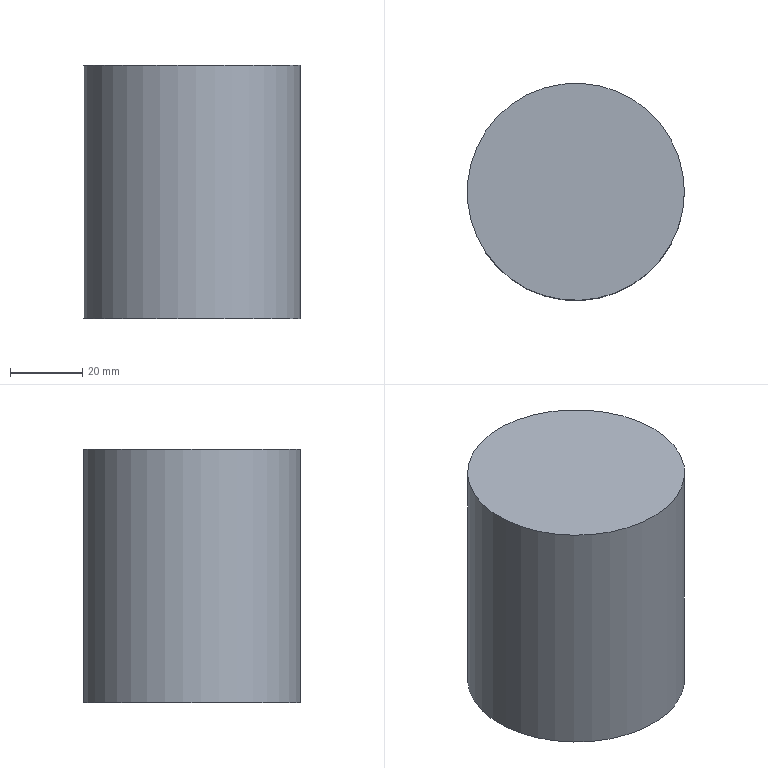Part | NX | features solid 2 | 1 solid | 3 faces | box 60 x 60 x 70 mm | volume 197920 mm3 | plane 2 | cylinder 1 | commonest cylinder face diameters 60 x1
STEP:
#1=CARTESIAN_POINT('',(-1275.,710.,-20.));
#2=VERTEX_POINT('',#1);
#3=CARTESIAN_POINT('',(-1305.,710.,-20.));
#4=DIRECTION('',(0.,0.,-1.));
#5=DIRECTION('',(1.,0.,0.));
#6=AXIS2_PLACEMENT_3D('',#3,#4,#5);
#7=CIRCLE('',#6,30.);
#8=EDGE_CURVE('',#2,#2,#7,.F.);
#9=ORIENTED_EDGE('',*,*,#8,.F.);
#10=EDGE_LOOP('',(#9));
#11=FACE_BOUND('',#10,.T.);
#12=CARTESIAN_POINT('',(-1275.,710.,-90.));
#13=VERTEX_POINT('',#12);
#14=CARTESIAN_POINT('',(-1305.,710.,-90.));
#15=DIRECTION('',(0.,0.,-1.));
#16=DIRECTION('',(1.,0.,0.));
#17=AXIS2_PLACEMENT_3D('',#14,#15,#16);
#18=CIRCLE('',#17,30.);
#19=EDGE_CURVE('',#13,#13,#18,.F.);
#20=ORIENTED_EDGE('',*,*,#19,.T.);
#21=EDGE_LOOP('',(#20));
#22=FACE_BOUND('',#21,.T.);
#23=CARTESIAN_POINT('',(-1305.,710.,-20.));
#24=DIRECTION('',(0.,0.,-1.));
#25=DIRECTION('',(1.,0.,0.));
#26=AXIS2_PLACEMENT_3D('',#23,#24,#25);
#27=CYLINDRICAL_SURFACE('',#26,30.);
#28=ADVANCED_FACE('',(#11,#22),#27,.T.);
#29=ORIENTED_EDGE('',*,*,#8,.T.);
#30=EDGE_LOOP('',(#29));
#31=FACE_BOUND('',#30,.T.);
#32=CARTESIAN_POINT('',(-1305.,710.,-20.));
#33=DIRECTION('',(0.,0.,1.));
#34=DIRECTION('',(1.,0.,0.));
#35=AXIS2_PLACEMENT_3D('',#32,#33,#34);
#36=PLANE('',#35);
#37=ADVANCED_FACE('',(#31),#36,.T.);
#38=ORIENTED_EDGE('',*,*,#19,.F.);
#39=EDGE_LOOP('',(#38));
#40=FACE_BOUND('',#39,.T.);
#41=CARTESIAN_POINT('',(-1305.,710.,-90.));
#42=DIRECTION('',(0.,0.,1.));
#43=DIRECTION('',(1.,0.,0.));
#44=AXIS2_PLACEMENT_3D('',#41,#42,#43);
#45=PLANE('',#44);
#46=ADVANCED_FACE('',(#40),#45,.F.);
#47=CLOSED_SHELL('',(#28,#37,#46));
#48=MANIFOLD_SOLID_BREP('',#47);
#49=(LENGTH_UNIT()NAMED_UNIT(*)SI_UNIT(.MILLI.,.METRE.));
#50=UNCERTAINTY_MEASURE_WITH_UNIT(LENGTH_MEASURE(0.00001),#49,'','');
#51=(NAMED_UNIT(*)PLANE_ANGLE_UNIT()SI_UNIT($,.RADIAN.));
#52=(NAMED_UNIT(*)SI_UNIT($,.STERADIAN.)SOLID_ANGLE_UNIT());
#53=(GEOMETRIC_REPRESENTATION_CONTEXT(3)GLOBAL_UNCERTAINTY_ASSIGNED_CONTEXT((#50))GLOBAL_UNIT_ASSIGNED_CONTEXT((#49,#51,#52))REPRESENTATION_CONTEXT('',''));
#54=ADVANCED_BREP_SHAPE_REPRESENTATION('',(#48),#53);